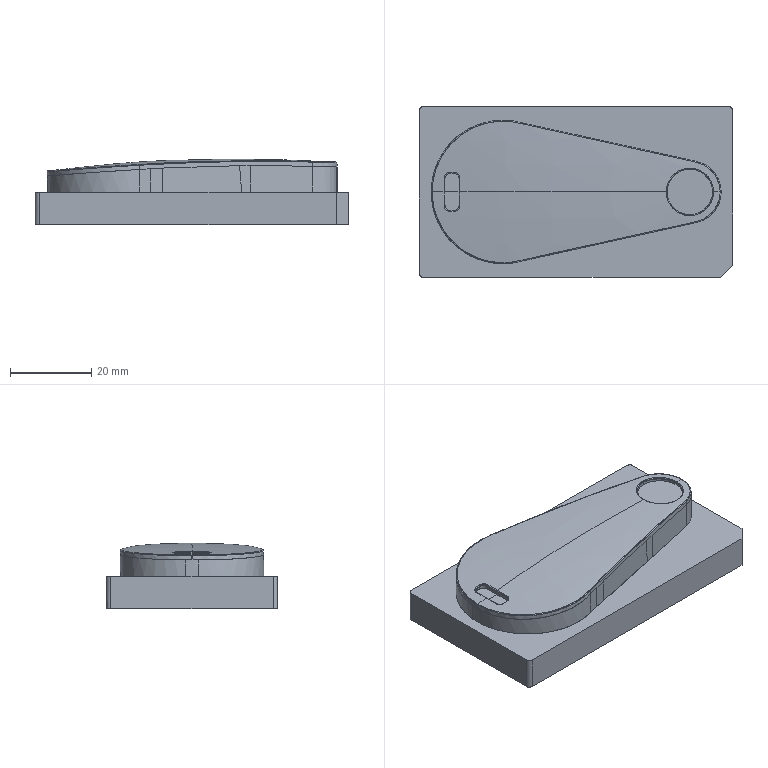CAM job | PowerMill | 3-axis milling, other | part box 77 x 42 x 16.114 mm
Tools:
number,name,type,diameter,tip_radius,length,cutting_length,overhang,flutes,holder,toolpaths_using
1,D10C,end_mill,10.0,0.0,60.0,,30.0,1,D42L35,2
2,D4C,end_mill,4.0,0.0,30.0,,15.0,1,D42L35,2
1,D10C_1_1,end_mill,10.0,0.0,60.0,,16.48,1,D42L35,6
2,D4C_1_1,end_mill,4.0,0.0,30.0,,8.32,1,D42L35,3
28,D2C_1_1,end_mill,2.0,0.0,3.0,,3.12,1,D42L35,2
3,D10_1_1,end_mill,10.0,0.0,60.0,,16.2,1,D42L35,6
7,R2_1_1_1,ball_nosed,4.0,2.0,30.0,,5.56,1,D42L35,2
12,D2_1_1,end_mill,2.0,0.0,3.0,,3.28,1,D42L35,2
6,R0.5_1_1,ball_nosed,1.0,0.5,3.0,,2.76,1,D42L35,1
13,Text_D4_1_1,taper_spherical,4.0,0.3,60.0,,8.36,1,D42L35,2
2,D4C_2_1,end_mill,4.0,0.0,30.0,,8.16,1,D42L35,3
7,R2_2_1,ball_nosed,4.0,2.0,30.0,,5.4,1,D42L35,2
6,R0.5_2_1,ball_nosed,1.0,0.5,3.0,,2.6,1,D42L35,1
Operations:
program,toolpath,strategy,tool,tool_number,tool_diameter,tip_radius,flutes,spindle_rpm,feed_cut,surface_speed_m_min_computed,feed_per_tooth_computed,tolerance,thickness,stepover,stepdown,cut_length,cut_time_min,total_time_min,workplane
29-B01-6-F,精公开粗01-扫面平行-D10C,raster_area_clear,D10C_1_1,1,10.0,0.0,1.0,8000.0,10000.0,251.33,1.25,0.03,0.28,6.0,1.0,1581.2,0.158,0.1675,
29-B01-6-F,精公开粗01-外形偏置-D10C,offset_area_clear,D10C_1_1,1,10.0,0.0,1.0,8000.0,10000.0,251.33,1.25,0.03,0.28,6.0,1.0,13333.434,1.333,1.388,
29-B01-6-F,精公开粗01-基准台等高-D10C,constantz,D10C_1_1,1,10.0,0.0,1.0,8000.0,10000.0,251.33,1.25,0.03,0.07,5.0,0.4,5868.98,0.587,0.5984,
29-B01-6-F,精公再粗02-外形偏置-D4C,offset_area_clear,D4C_1_1,2,4.0,0.0,1.0,18000.0,6000.0,226.19,0.3333,0.03,0.0,2.0,1.0,8052.892,1.342,1.386,
29-B01-6-F,精公再粗02-平行中光-D4C,raster,D4C_1_1,2,4.0,0.0,1.0,18000.0,6000.0,226.19,0.3333,0.03,0.0,0.2,1.0,10219.727,1.703,1.73,
29-B01-6-F,精公再粗02-平坦面平行-D4C,raster_area_clear,D4C_1_1,2,4.0,0.0,1.0,18000.0,3000.0,226.19,0.1667,0.03,0.0,2.0,1.0,46.131,0.015,0.0289,
29-B01-6-F,精公再粗03-外形偏置-D2C,offset_area_clear,D2C_1_1,28,2.0,0.0,1.0,18000.0,4000.0,113.1,0.2222,0.03,0.0,1.1,1.0,142.187,0.035,0.0857,
29-B01-6-F,精公基准台01-基准面偏置-D10,offset_area_clear,D10_1_1,3,10.0,0.0,1.0,8500.0,600.0,267.04,0.0706,0.005,0.38,5.0,1.0,372.433,0.621,0.6413,
29-B01-6-F,精公基准台01-外形侧光-D10,profile_area_clear,D10_1_1,3,10.0,0.0,1.0,8500.0,600.0,267.04,0.0706,0.005,-0.07,0.08,1.0,409.591,0.683,0.7038,
29-B01-6-F,精公基准台01-基准台侧光-D10,profile_area_clear,D10_1_1,3,10.0,0.0,1.0,8500.0,600.0,267.04,0.0706,0.005,0.0,0.08,1.0,533.233,0.889,0.9548,
29-B01-6-F,精公精光01-平行-R2,raster,R2_1_1_1,7,4.0,2.0,1.0,18000.0,2000.0,226.19,0.1111,0.005,-0.075,0.05,1.0,43572.739,21.786,21.852,
29-B01-6-F,精公精光02-等高-R2,constantz,R2_1_1_1,7,4.0,2.0,1.0,18000.0,2000.0,226.19,0.1111,0.005,-0.075,5.0,0.05,5759.994,2.88,3.15,
29-B01-6-F,精公精光03-等高-D2,constantz,D2_1_1,12,2.0,0.0,1.0,18000.0,1500.0,113.1,0.0833,0.005,-0.075,5.0,0.03,1874.321,1.25,1.399,
29-B01-6-F,精公精光04-三维偏置-R0.5,offset_3d,R0.5_1_1,6,1.0,0.5,1.0,20000.0,1000.0,62.83,0.05,0.005,-0.075,0.02,1.0,2249.112,2.249,2.28,
29-B01-6-F,精公刻字01-刻字-Text_D4,pattern,Text_D4_1_1,13,4.0,0.3,1.0,15000.0,1000.0,188.5,0.0667,0.005,0.0,5.0,1.0,76.198,0.076,0.0954,
29-B01-6-R,粗公开粗01-扫面平行-D10C,raster_area_clear,D10C_1_1,1,10.0,0.0,1.0,8000.0,10000.0,251.33,1.25,0.03,0.15,6.0,1.0,1576.0,0.158,0.167,
29-B01-6-R,粗公开粗01-外形偏置-D10C,offset_area_clear,D10C_1_1,1,10.0,0.0,1.0,8000.0,10000.0,251.33,1.25,0.03,0.15,6.0,1.0,12678.583,1.268,1.321,
29-B01-6-R,粗公开粗01-基准台等高-D10C,constantz,D10C_1_1,1,10.0,0.0,1.0,8000.0,10000.0,251.33,1.25,0.03,0.07,5.0,0.4,5868.98,0.587,0.5984,
29-B01-6-R,粗公再粗02-外形偏置-D4C,offset_area_clear,D4C_2_1,2,4.0,0.0,1.0,18000.0,6000.0,226.19,0.3333,0.03,-0.13,2.0,1.0,7243.686,1.207,1.253,
29-B01-6-R,粗公再粗02-平行中光-D4C,raster,D4C_2_1,2,4.0,0.0,1.0,18000.0,6000.0,226.19,0.3333,0.03,-0.13,0.2,1.0,10063.581,1.677,1.707,
29-B01-6-R,粗公再粗02-平坦面平行-D4C,raster_area_clear,D4C_2_1,2,4.0,0.0,1.0,18000.0,3000.0,226.19,0.1667,0.03,-0.13,2.0,1.0,47.794,0.016,0.0296,
29-B01-6-R,粗公再粗03-外形偏置-D2C,offset_area_clear,D2C_1_1,28,2.0,0.0,1.0,18000.0,4000.0,113.1,0.2222,0.03,-0.13,1.1,1.0,148.654,0.037,0.0879,
29-B01-6-R,粗公基准台01-基准面偏置-D10,offset_area_clear,D10_1_1,3,10.0,0.0,1.0,8500.0,600.0,267.04,0.0706,0.01,0.25,5.0,1.0,370.543,0.617,0.6381,
29-B01-6-R,粗公基准台01-外形侧光-D10,profile_area_clear,D10_1_1,3,10.0,0.0,1.0,8500.0,600.0,267.04,0.0706,0.01,-0.2,0.08,1.0,407.955,0.68,0.7011,
29-B01-6-R,粗公基准台01-基准台侧光-D10,profile_area_clear,D10_1_1,3,10.0,0.0,1.0,8500.0,600.0,267.04,0.0706,0.01,0.0,0.08,1.0,533.217,0.889,0.9547,
29-B01-6-R,粗公精光01-平行-R2,raster,R2_2_1,7,4.0,2.0,1.0,18000.0,2000.0,226.19,0.1111,0.01,-0.205,0.06,1.0,35432.315,17.716,17.78,
29-B01-6-R,粗公精光02-等高-R2,constantz,R2_2_1,7,4.0,2.0,1.0,18000.0,2000.0,226.19,0.1111,0.01,-0.205,5.0,0.06,4333.836,2.167,2.402,
29-B01-6-R,粗公精光03-等高-D2,constantz,D2_1_1,12,2.0,0.0,1.0,18000.0,1500.0,113.1,0.0833,0.01,-0.205,5.0,0.036,1621.021,1.081,1.2,
29-B01-6-R,粗公精光04-三维偏置-R0.5,offset_3d,R0.5_2_1,6,1.0,0.5,1.0,20000.0,1000.0,62.83,0.05,0.01,-0.205,0.024,1.0,1391.06,1.391,1.417,
29-B01-6-R,粗公刻字01-刻字-Text_D4,pattern,Text_D4_1_1,13,4.0,0.3,1.0,15000.0,1000.0,188.5,0.0667,0.01,0.0,5.0,1.0,74.473,0.074,0.0928,
,精公开粗01-外形偏置-D10C_Reference,offset_area_clear,D10C,1,10.0,0.0,1.0,8000.0,10000.0,251.33,1.25,0.03,0.28,6.0,1.0,26184.44,2.618,2.722,
,精公再粗02-外形偏置-D4C_Reference,offset_area_clear,D4C,2,4.0,0.0,1.0,18000.0,6000.0,226.19,0.3333,0.03,0.0,2.0,1.0,15284.624,2.547,2.635,
,粗公开粗01-外形偏置-D10C_Reference,offset_area_clear,D10C,1,10.0,0.0,1.0,8000.0,10000.0,251.33,1.25,0.03,0.15,6.0,1.0,25473.146,2.547,2.648,
,粗公再粗02-外形偏置-D4C_Reference,offset_area_clear,D4C,2,4.0,0.0,1.0,18000.0,6000.0,226.19,0.3333,0.03,-0.13,2.0,1.0,14454.992,2.409,2.494,